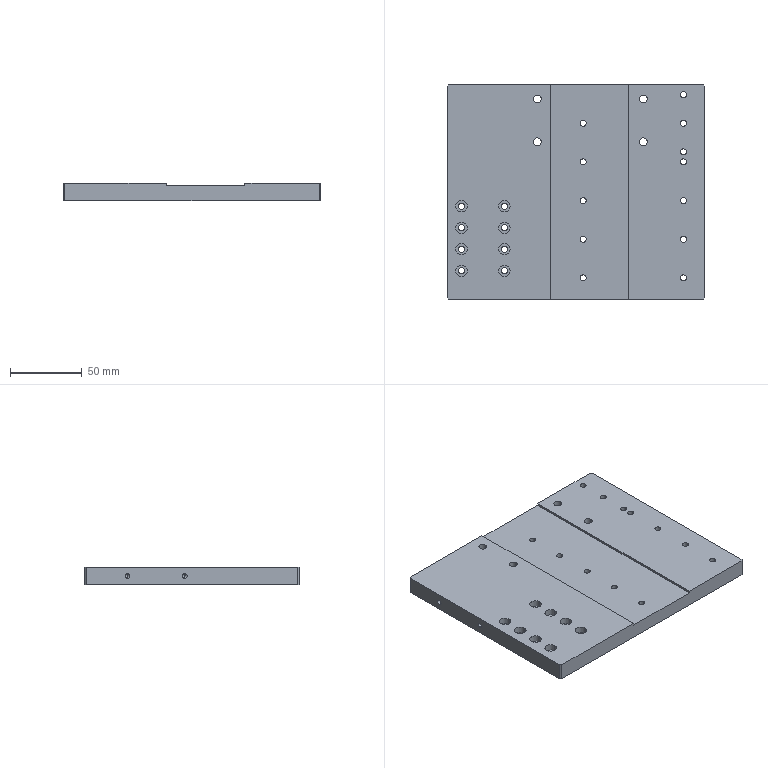Part | STEP file | Z-axis assembly mounting plate | 1 solid | 114 faces | box 180 x 150 x 12 mm | volume 304023 mm3 | cylinder 80 | plane 26 | cone 8 | commonest cylinder face diameters 4.2 x24 4.5 x16 8 x16 3.3 x8 5.5 x8 10 x8